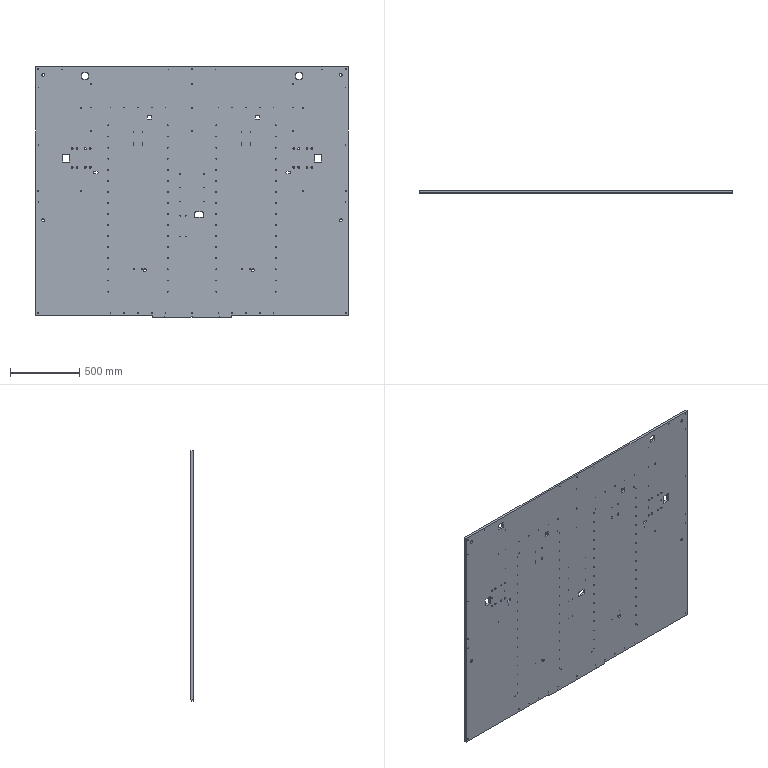Part | STEP file | 1 solid | 537 faces | box 2260 x 16 x 1812 mm | volume 64799622 mm3 | cylinder 421 | cone 74 | plane 42 | commonest cylinder face diameters 6.8 x128 4.2 x98 10 x52 5 x40 12 x32 9 x25